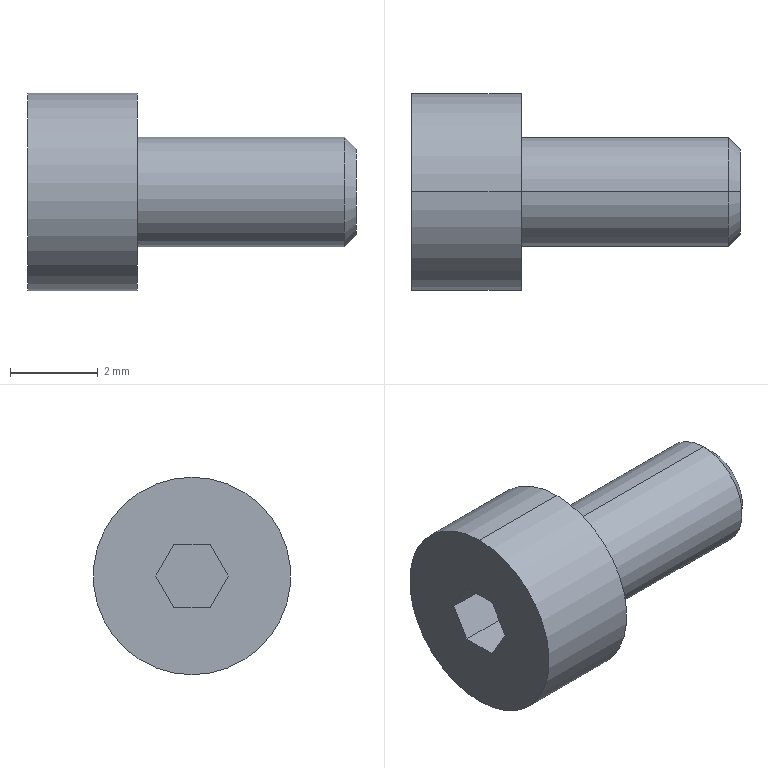Part | STEP file | _DBA11-D25-d10-e12-005.stp | 1 solid | 16 faces | box 7.5 x 4.5 x 4.5 mm | volume 61.818 mm3 | plane 10 | cylinder 4 | cone 2 | commonest cylinder face diameters 2.5 x2 4.5 x2
STEP:
#1=CARTESIAN_POINT('',(2.5,0.,-1.25));
#2=VERTEX_POINT('',#1);
#3=CARTESIAN_POINT('',(2.5,0.,1.25));
#4=VERTEX_POINT('',#3);
#5=CARTESIAN_POINT('',(2.5,0.,0.));
#6=DIRECTION('',(-1.,0.,0.));
#7=DIRECTION('',(0.,0.,1.));
#8=AXIS2_PLACEMENT_3D('',#5,#6,#7);
#9=CIRCLE('',#8,1.25);
#10=EDGE_CURVE('',#2,#4,#9,.T.);
#11=ORIENTED_EDGE('',*,*,#10,.F.);
#12=CARTESIAN_POINT('',(7.224,0.,-1.25));
#13=VERTEX_POINT('',#12);
#14=CARTESIAN_POINT('',(0.,0.,-1.25));
#15=DIRECTION('',(1.,0.,0.));
#16=VECTOR('',#15,1000.);
#17=LINE('',#14,#16);
#18=EDGE_CURVE('',#2,#13,#17,.T.);
#19=ORIENTED_EDGE('',*,*,#18,.T.);
#20=CARTESIAN_POINT('',(7.224,0.,1.25));
#21=VERTEX_POINT('',#20);
#22=CARTESIAN_POINT('',(7.224,0.,0.));
#23=DIRECTION('',(-1.,0.,0.));
#24=DIRECTION('',(0.,0.,1.));
#25=AXIS2_PLACEMENT_3D('',#22,#23,#24);
#26=CIRCLE('',#25,1.25);
#27=EDGE_CURVE('',#13,#21,#26,.T.);
#28=ORIENTED_EDGE('',*,*,#27,.T.);
#29=CARTESIAN_POINT('',(0.,0.,1.25));
#30=DIRECTION('',(1.,0.,0.));
#31=VECTOR('',#30,1000.);
#32=LINE('',#29,#31);
#33=EDGE_CURVE('',#4,#21,#32,.T.);
#34=ORIENTED_EDGE('',*,*,#33,.F.);
#35=EDGE_LOOP('',(#11,#19,#28,#34));
#36=FACE_OUTER_BOUND('',#35,.T.);
#37=CARTESIAN_POINT('',(0.,0.,0.));
#38=DIRECTION('',(1.,0.,0.));
#39=DIRECTION('',(0.,0.,1.));
#40=AXIS2_PLACEMENT_3D('',#37,#38,#39);
#41=CYLINDRICAL_SURFACE('',#40,1.25);
#42=ADVANCED_FACE('',(#36),#41,.T.);
#43=CARTESIAN_POINT('',(0.,0.,-2.25));
#44=VERTEX_POINT('',#43);
#45=CARTESIAN_POINT('',(0.,0.,2.25));
#46=VERTEX_POINT('',#45);
#47=CARTESIAN_POINT('',(0.,0.,0.));
#48=DIRECTION('',(-1.,0.,0.));
#49=DIRECTION('',(0.,0.,1.));
#50=AXIS2_PLACEMENT_3D('',#47,#48,#49);
#51=CIRCLE('',#50,2.25);
#52=EDGE_CURVE('',#44,#46,#51,.T.);
#53=ORIENTED_EDGE('',*,*,#52,.F.);
#54=CARTESIAN_POINT('',(2.5,0.,-2.25));
#55=VERTEX_POINT('',#54);
#56=CARTESIAN_POINT('',(0.,0.,-2.25));
#57=DIRECTION('',(1.,0.,0.));
#58=VECTOR('',#57,1000.);
#59=LINE('',#56,#58);
#60=EDGE_CURVE('',#44,#55,#59,.T.);
#61=ORIENTED_EDGE('',*,*,#60,.T.);
#62=CARTESIAN_POINT('',(2.5,0.,2.25));
#63=VERTEX_POINT('',#62);
#64=CARTESIAN_POINT('',(2.5,0.,0.));
#65=DIRECTION('',(-1.,0.,0.));
#66=DIRECTION('',(0.,0.,1.));
#67=AXIS2_PLACEMENT_3D('',#64,#65,#66);
#68=CIRCLE('',#67,2.25);
#69=EDGE_CURVE('',#55,#63,#68,.T.);
#70=ORIENTED_EDGE('',*,*,#69,.T.);
#71=CARTESIAN_POINT('',(0.,0.,2.25));
#72=DIRECTION('',(1.,0.,0.));
#73=VECTOR('',#72,1000.);
#74=LINE('',#71,#73);
#75=EDGE_CURVE('',#46,#63,#74,.T.);
#76=ORIENTED_EDGE('',*,*,#75,.F.);
#77=EDGE_LOOP('',(#53,#61,#70,#76));
#78=FACE_OUTER_BOUND('',#77,.T.);
#79=CARTESIAN_POINT('',(0.,0.,0.));
#80=DIRECTION('',(1.,0.,0.));
#81=DIRECTION('',(0.,0.,1.));
#82=AXIS2_PLACEMENT_3D('',#79,#80,#81);
#83=CYLINDRICAL_SURFACE('',#82,2.25);
#84=ADVANCED_FACE('',(#78),#83,.T.);
#85=CARTESIAN_POINT('',(7.5,0.,0.974));
#86=VERTEX_POINT('',#85);
#87=CARTESIAN_POINT('',(7.5,0.,-0.974));
#88=VERTEX_POINT('',#87);
#89=CARTESIAN_POINT('',(7.5,0.,0.));
#90=DIRECTION('',(-1.,0.,0.));
#91=DIRECTION('',(0.,0.,1.));
#92=AXIS2_PLACEMENT_3D('',#89,#90,#91);
#93=CIRCLE('',#92,0.974);
#94=EDGE_CURVE('',#86,#88,#93,.T.);
#95=ORIENTED_EDGE('',*,*,#94,.T.);
#96=CARTESIAN_POINT('',(7.5,0.,-0.974));
#97=DIRECTION('',(-0.7071,0.,-0.7071));
#98=VECTOR('',#97,1000.);
#99=LINE('',#96,#98);
#100=EDGE_CURVE('',#88,#13,#99,.T.);
#101=ORIENTED_EDGE('',*,*,#100,.T.);
#102=CARTESIAN_POINT('',(7.224,0.,0.));
#103=DIRECTION('',(-1.,0.,0.));
#104=DIRECTION('',(0.,0.,1.));
#105=AXIS2_PLACEMENT_3D('',#102,#103,#104);
#106=CIRCLE('',#105,1.25);
#107=EDGE_CURVE('',#21,#13,#106,.T.);
#108=ORIENTED_EDGE('',*,*,#107,.F.);
#109=CARTESIAN_POINT('',(7.5,0.,0.974));
#110=DIRECTION('',(-0.7071,0.,0.7071));
#111=VECTOR('',#110,1000.);
#112=LINE('',#109,#111);
#113=EDGE_CURVE('',#86,#21,#112,.T.);
#114=ORIENTED_EDGE('',*,*,#113,.F.);
#115=EDGE_LOOP('',(#95,#101,#108,#114));
#116=FACE_OUTER_BOUND('',#115,.T.);
#117=CARTESIAN_POINT('',(7.5,0.,0.));
#118=DIRECTION('',(-1.,0.,0.));
#119=DIRECTION('',(0.,0.,1.));
#120=AXIS2_PLACEMENT_3D('',#117,#118,#119);
#121=CONICAL_SURFACE('',#120,0.974,0.7854);
#122=ADVANCED_FACE('',(#116),#121,.T.);
#123=ORIENTED_EDGE('',*,*,#100,.F.);
#124=CARTESIAN_POINT('',(7.5,0.,0.));
#125=DIRECTION('',(-1.,0.,0.));
#126=DIRECTION('',(0.,0.,1.));
#127=AXIS2_PLACEMENT_3D('',#124,#125,#126);
#128=CIRCLE('',#127,0.974);
#129=EDGE_CURVE('',#88,#86,#128,.T.);
#130=ORIENTED_EDGE('',*,*,#129,.T.);
#131=ORIENTED_EDGE('',*,*,#113,.T.);
#132=ORIENTED_EDGE('',*,*,#27,.F.);
#133=EDGE_LOOP('',(#123,#130,#131,#132));
#134=FACE_OUTER_BOUND('',#133,.T.);
#135=CARTESIAN_POINT('',(7.5,0.,0.));
#136=DIRECTION('',(-1.,0.,0.));
#137=DIRECTION('',(0.,0.,1.));
#138=AXIS2_PLACEMENT_3D('',#135,#136,#137);
#139=CONICAL_SURFACE('',#138,0.974,0.7854);
#140=ADVANCED_FACE('',(#134),#139,.T.);
#141=ORIENTED_EDGE('',*,*,#94,.F.);
#142=ORIENTED_EDGE('',*,*,#129,.F.);
#143=EDGE_LOOP('',(#141,#142));
#144=FACE_OUTER_BOUND('',#143,.T.);
#145=CARTESIAN_POINT('',(7.5,0.,0.));
#146=DIRECTION('',(-1.,0.,0.));
#147=DIRECTION('',(0.,0.,1.));
#148=AXIS2_PLACEMENT_3D('',#145,#146,#147);
#149=PLANE('',#148);
#150=ADVANCED_FACE('',(#144),#149,.F.);
#151=CARTESIAN_POINT('',(0.,0.,0.));
#152=DIRECTION('',(-1.,0.,0.));
#153=DIRECTION('',(0.,0.,1.));
#154=AXIS2_PLACEMENT_3D('',#151,#152,#153);
#155=CIRCLE('',#154,2.25);
#156=EDGE_CURVE('',#46,#44,#155,.T.);
#157=ORIENTED_EDGE('',*,*,#156,.T.);
#158=ORIENTED_EDGE('',*,*,#52,.T.);
#159=EDGE_LOOP('',(#157,#158));
#160=FACE_OUTER_BOUND('',#159,.T.);
#161=CARTESIAN_POINT('',(0.,-0.4124,0.7143));
#162=VERTEX_POINT('',#161);
#163=CARTESIAN_POINT('',(0.,-0.8248,0.));
#164=VERTEX_POINT('',#163);
#165=CARTESIAN_POINT('',(0.,-0.4124,0.7143));
#166=DIRECTION('',(0.,-0.5,-0.866));
#167=VECTOR('',#166,1000.);
#168=LINE('',#165,#167);
#169=EDGE_CURVE('',#162,#164,#168,.T.);
#170=ORIENTED_EDGE('',*,*,#169,.T.);
#171=CARTESIAN_POINT('',(0.,-0.4124,-0.7143));
#172=VERTEX_POINT('',#171);
#173=CARTESIAN_POINT('',(0.,-0.8248,0.));
#174=DIRECTION('',(0.,0.5,-0.866));
#175=VECTOR('',#174,1000.);
#176=LINE('',#173,#175);
#177=EDGE_CURVE('',#164,#172,#176,.T.);
#178=ORIENTED_EDGE('',*,*,#177,.T.);
#179=CARTESIAN_POINT('',(0.,0.4124,-0.7143));
#180=VERTEX_POINT('',#179);
#181=CARTESIAN_POINT('',(0.,-0.4124,-0.7143));
#182=DIRECTION('',(0.,1.,0.));
#183=VECTOR('',#182,1000.);
#184=LINE('',#181,#183);
#185=EDGE_CURVE('',#172,#180,#184,.T.);
#186=ORIENTED_EDGE('',*,*,#185,.T.);
#187=CARTESIAN_POINT('',(0.,0.8248,0.));
#188=VERTEX_POINT('',#187);
#189=CARTESIAN_POINT('',(0.,0.4124,-0.7143));
#190=DIRECTION('',(0.,0.5,0.866));
#191=VECTOR('',#190,1000.);
#192=LINE('',#189,#191);
#193=EDGE_CURVE('',#180,#188,#192,.T.);
#194=ORIENTED_EDGE('',*,*,#193,.T.);
#195=CARTESIAN_POINT('',(0.,0.4124,0.7143));
#196=VERTEX_POINT('',#195);
#197=CARTESIAN_POINT('',(0.,0.8248,0.));
#198=DIRECTION('',(0.,-0.5,0.866));
#199=VECTOR('',#198,1000.);
#200=LINE('',#197,#199);
#201=EDGE_CURVE('',#188,#196,#200,.T.);
#202=ORIENTED_EDGE('',*,*,#201,.T.);
#203=CARTESIAN_POINT('',(0.,0.4124,0.7143));
#204=DIRECTION('',(0.,-1.,0.));
#205=VECTOR('',#204,1000.);
#206=LINE('',#203,#205);
#207=EDGE_CURVE('',#196,#162,#206,.T.);
#208=ORIENTED_EDGE('',*,*,#207,.T.);
#209=EDGE_LOOP('',(#170,#178,#186,#194,#202,#208));
#210=FACE_BOUND('',#209,.T.);
#211=CARTESIAN_POINT('',(0.,-2.25,0.));
#212=DIRECTION('',(1.,0.,0.));
#213=DIRECTION('',(0.,1.,0.));
#214=AXIS2_PLACEMENT_3D('',#211,#212,#213);
#215=PLANE('',#214);
#216=ADVANCED_FACE('',(#160,#210),#215,.F.);
#217=ORIENTED_EDGE('',*,*,#60,.F.);
#218=ORIENTED_EDGE('',*,*,#156,.F.);
#219=ORIENTED_EDGE('',*,*,#75,.T.);
#220=CARTESIAN_POINT('',(2.5,0.,0.));
#221=DIRECTION('',(-1.,0.,0.));
#222=DIRECTION('',(0.,0.,1.));
#223=AXIS2_PLACEMENT_3D('',#220,#221,#222);
#224=CIRCLE('',#223,2.25);
#225=EDGE_CURVE('',#63,#55,#224,.T.);
#226=ORIENTED_EDGE('',*,*,#225,.T.);
#227=EDGE_LOOP('',(#217,#218,#219,#226));
#228=FACE_OUTER_BOUND('',#227,.T.);
#229=CARTESIAN_POINT('',(0.,0.,0.));
#230=DIRECTION('',(1.,0.,0.));
#231=DIRECTION('',(0.,0.,1.));
#232=AXIS2_PLACEMENT_3D('',#229,#230,#231);
#233=CYLINDRICAL_SURFACE('',#232,2.25);
#234=ADVANCED_FACE('',(#228),#233,.T.);
#235=ORIENTED_EDGE('',*,*,#225,.F.);
#236=ORIENTED_EDGE('',*,*,#69,.F.);
#237=EDGE_LOOP('',(#235,#236));
#238=FACE_OUTER_BOUND('',#237,.T.);
#239=CARTESIAN_POINT('',(2.5,0.,0.));
#240=DIRECTION('',(-1.,0.,0.));
#241=DIRECTION('',(0.,0.,1.));
#242=AXIS2_PLACEMENT_3D('',#239,#240,#241);
#243=CIRCLE('',#242,1.25);
#244=EDGE_CURVE('',#4,#2,#243,.T.);
#245=ORIENTED_EDGE('',*,*,#244,.T.);
#246=ORIENTED_EDGE('',*,*,#10,.T.);
#247=EDGE_LOOP('',(#245,#246));
#248=FACE_BOUND('',#247,.T.);
#249=CARTESIAN_POINT('',(2.5,-1.25,0.));
#250=DIRECTION('',(-1.,0.,0.));
#251=DIRECTION('',(0.,0.,1.));
#252=AXIS2_PLACEMENT_3D('',#249,#250,#251);
#253=PLANE('',#252);
#254=ADVANCED_FACE('',(#238,#248),#253,.F.);
#255=ORIENTED_EDGE('',*,*,#18,.F.);
#256=ORIENTED_EDGE('',*,*,#244,.F.);
#257=ORIENTED_EDGE('',*,*,#33,.T.);
#258=ORIENTED_EDGE('',*,*,#107,.T.);
#259=EDGE_LOOP('',(#255,#256,#257,#258));
#260=FACE_OUTER_BOUND('',#259,.T.);
#261=CARTESIAN_POINT('',(0.,0.,0.));
#262=DIRECTION('',(1.,0.,0.));
#263=DIRECTION('',(0.,0.,1.));
#264=AXIS2_PLACEMENT_3D('',#261,#262,#263);
#265=CYLINDRICAL_SURFACE('',#264,1.25);
#266=ADVANCED_FACE('',(#260),#265,.T.);
#267=ORIENTED_EDGE('',*,*,#207,.F.);
#268=CARTESIAN_POINT('',(1.25,0.4124,0.7143));
#269=VERTEX_POINT('',#268);
#270=CARTESIAN_POINT('',(1.25,0.4124,0.7143));
#271=DIRECTION('',(-1.,0.,0.));
#272=VECTOR('',#271,1000.);
#273=LINE('',#270,#272);
#274=EDGE_CURVE('',#269,#196,#273,.T.);
#275=ORIENTED_EDGE('',*,*,#274,.F.);
#276=CARTESIAN_POINT('',(1.25,-0.4124,0.7143));
#277=VERTEX_POINT('',#276);
#278=CARTESIAN_POINT('',(1.25,0.4124,0.7143));
#279=DIRECTION('',(0.,-1.,0.));
#280=VECTOR('',#279,1000.);
#281=LINE('',#278,#280);
#282=EDGE_CURVE('',#269,#277,#281,.T.);
#283=ORIENTED_EDGE('',*,*,#282,.T.);
#284=CARTESIAN_POINT('',(1.25,-0.4124,0.7143));
#285=DIRECTION('',(-1.,0.,0.));
#286=VECTOR('',#285,1000.);
#287=LINE('',#284,#286);
#288=EDGE_CURVE('',#277,#162,#287,.T.);
#289=ORIENTED_EDGE('',*,*,#288,.T.);
#290=EDGE_LOOP('',(#267,#275,#283,#289));
#291=FACE_OUTER_BOUND('',#290,.T.);
#292=CARTESIAN_POINT('',(1.25,0.4124,0.7143));
#293=DIRECTION('',(0.,0.,-1.));
#294=DIRECTION('',(0.,-1.,0.));
#295=AXIS2_PLACEMENT_3D('',#292,#293,#294);
#296=PLANE('',#295);
#297=ADVANCED_FACE('',(#291),#296,.T.);
#298=ORIENTED_EDGE('',*,*,#169,.F.);
#299=ORIENTED_EDGE('',*,*,#288,.F.);
#300=CARTESIAN_POINT('',(1.25,-0.8248,0.));
#301=VERTEX_POINT('',#300);
#302=CARTESIAN_POINT('',(1.25,-0.4124,0.7143));
#303=DIRECTION('',(0.,-0.5,-0.866));
#304=VECTOR('',#303,1000.);
#305=LINE('',#302,#304);
#306=EDGE_CURVE('',#277,#301,#305,.T.);
#307=ORIENTED_EDGE('',*,*,#306,.T.);
#308=CARTESIAN_POINT('',(1.25,-0.8248,0.));
#309=DIRECTION('',(-1.,0.,0.));
#310=VECTOR('',#309,1000.);
#311=LINE('',#308,#310);
#312=EDGE_CURVE('',#301,#164,#311,.T.);
#313=ORIENTED_EDGE('',*,*,#312,.T.);
#314=EDGE_LOOP('',(#298,#299,#307,#313));
#315=FACE_OUTER_BOUND('',#314,.T.);
#316=CARTESIAN_POINT('',(1.25,-0.4124,0.7143));
#317=DIRECTION('',(0.,0.866,-0.5));
#318=DIRECTION('',(-1.,0.,0.));
#319=AXIS2_PLACEMENT_3D('',#316,#317,#318);
#320=PLANE('',#319);
#321=ADVANCED_FACE('',(#315),#320,.T.);
#322=ORIENTED_EDGE('',*,*,#177,.F.);
#323=ORIENTED_EDGE('',*,*,#312,.F.);
#324=CARTESIAN_POINT('',(1.25,-0.4124,-0.7143));
#325=VERTEX_POINT('',#324);
#326=CARTESIAN_POINT('',(1.25,-0.8248,0.));
#327=DIRECTION('',(0.,0.5,-0.866));
#328=VECTOR('',#327,1000.);
#329=LINE('',#326,#328);
#330=EDGE_CURVE('',#301,#325,#329,.T.);
#331=ORIENTED_EDGE('',*,*,#330,.T.);
#332=CARTESIAN_POINT('',(1.25,-0.4124,-0.7143));
#333=DIRECTION('',(-1.,0.,0.));
#334=VECTOR('',#333,1000.);
#335=LINE('',#332,#334);
#336=EDGE_CURVE('',#325,#172,#335,.T.);
#337=ORIENTED_EDGE('',*,*,#336,.T.);
#338=EDGE_LOOP('',(#322,#323,#331,#337));
#339=FACE_OUTER_BOUND('',#338,.T.);
#340=CARTESIAN_POINT('',(1.25,-0.8248,0.));
#341=DIRECTION('',(0.,0.866,0.5));
#342=DIRECTION('',(1.,0.,0.));
#343=AXIS2_PLACEMENT_3D('',#340,#341,#342);
#344=PLANE('',#343);
#345=ADVANCED_FACE('',(#339),#344,.T.);
#346=ORIENTED_EDGE('',*,*,#185,.F.);
#347=ORIENTED_EDGE('',*,*,#336,.F.);
#348=CARTESIAN_POINT('',(1.25,0.4124,-0.7143));
#349=VERTEX_POINT('',#348);
#350=CARTESIAN_POINT('',(1.25,-0.4124,-0.7143));
#351=DIRECTION('',(0.,1.,0.));
#352=VECTOR('',#351,1000.);
#353=LINE('',#350,#352);
#354=EDGE_CURVE('',#325,#349,#353,.T.);
#355=ORIENTED_EDGE('',*,*,#354,.T.);
#356=CARTESIAN_POINT('',(1.25,0.4124,-0.7143));
#357=DIRECTION('',(-1.,0.,0.));
#358=VECTOR('',#357,1000.);
#359=LINE('',#356,#358);
#360=EDGE_CURVE('',#349,#180,#359,.T.);
#361=ORIENTED_EDGE('',*,*,#360,.T.);
#362=EDGE_LOOP('',(#346,#347,#355,#361));
#363=FACE_OUTER_BOUND('',#362,.T.);
#364=CARTESIAN_POINT('',(1.25,-0.4124,-0.7143));
#365=DIRECTION('',(0.,0.,1.));
#366=DIRECTION('',(1.,0.,0.));
#367=AXIS2_PLACEMENT_3D('',#364,#365,#366);
#368=PLANE('',#367);
#369=ADVANCED_FACE('',(#363),#368,.T.);
#370=ORIENTED_EDGE('',*,*,#193,.F.);
#371=ORIENTED_EDGE('',*,*,#360,.F.);
#372=CARTESIAN_POINT('',(1.25,0.8248,0.));
#373=VERTEX_POINT('',#372);
#374=CARTESIAN_POINT('',(1.25,0.4124,-0.7143));
#375=DIRECTION('',(0.,0.5,0.866));
#376=VECTOR('',#375,1000.);
#377=LINE('',#374,#376);
#378=EDGE_CURVE('',#349,#373,#377,.T.);
#379=ORIENTED_EDGE('',*,*,#378,.T.);
#380=CARTESIAN_POINT('',(1.25,0.8248,0.));
#381=DIRECTION('',(-1.,0.,0.));
#382=VECTOR('',#381,1000.);
#383=LINE('',#380,#382);
#384=EDGE_CURVE('',#373,#188,#383,.T.);
#385=ORIENTED_EDGE('',*,*,#384,.T.);
#386=EDGE_LOOP('',(#370,#371,#379,#385));
#387=FACE_OUTER_BOUND('',#386,.T.);
#388=CARTESIAN_POINT('',(1.25,0.4124,-0.7143));
#389=DIRECTION('',(0.,-0.866,0.5));
#390=DIRECTION('',(-1.,0.,0.));
#391=AXIS2_PLACEMENT_3D('',#388,#389,#390);
#392=PLANE('',#391);
#393=ADVANCED_FACE('',(#387),#392,.T.);
#394=ORIENTED_EDGE('',*,*,#201,.F.);
#395=ORIENTED_EDGE('',*,*,#384,.F.);
#396=CARTESIAN_POINT('',(1.25,0.8248,0.));
#397=DIRECTION('',(0.,-0.5,0.866));
#398=VECTOR('',#397,1000.);
#399=LINE('',#396,#398);
#400=EDGE_CURVE('',#373,#269,#399,.T.);
#401=ORIENTED_EDGE('',*,*,#400,.T.);
#402=ORIENTED_EDGE('',*,*,#274,.T.);
#403=EDGE_LOOP('',(#394,#395,#401,#402));
#404=FACE_OUTER_BOUND('',#403,.T.);
#405=CARTESIAN_POINT('',(1.25,0.8248,0.));
#406=DIRECTION('',(0.,-0.866,-0.5));
#407=DIRECTION('',(0.,0.5,-0.866));
#408=AXIS2_PLACEMENT_3D('',#405,#406,#407);
#409=PLANE('',#408);
#410=ADVANCED_FACE('',(#404),#409,.T.);
#411=ORIENTED_EDGE('',*,*,#282,.F.);
#412=ORIENTED_EDGE('',*,*,#400,.F.);
#413=ORIENTED_EDGE('',*,*,#378,.F.);
#414=ORIENTED_EDGE('',*,*,#354,.F.);
#415=ORIENTED_EDGE('',*,*,#330,.F.);
#416=ORIENTED_EDGE('',*,*,#306,.F.);
#417=EDGE_LOOP('',(#411,#412,#413,#414,#415,#416));
#418=FACE_OUTER_BOUND('',#417,.T.);
#419=CARTESIAN_POINT('',(1.25,0.,0.));
#420=DIRECTION('',(1.,0.,0.));
#421=DIRECTION('',(0.,1.,0.));
#422=AXIS2_PLACEMENT_3D('',#419,#420,#421);
#423=PLANE('',#422);
#424=ADVANCED_FACE('',(#418),#423,.F.);
#425=CLOSED_SHELL('',(#42,#84,#122,#140,#150,#216,#234,#254,#266,#297,#321,#345,#369,#393,#410,#424));
#426=MANIFOLD_SOLID_BREP('',#425);
#427=CARTESIAN_POINT('',(0.,0.,0.));
#428=DIRECTION('',(0.,0.,1.));
#429=DIRECTION('',(1.,0.,0.));
#430=AXIS2_PLACEMENT_3D('',#427,#428,#429);
#431=(LENGTH_UNIT()NAMED_UNIT(*)SI_UNIT(.MILLI.,.METRE.));
#432=UNCERTAINTY_MEASURE_WITH_UNIT(LENGTH_MEASURE(0.00001),#431,'','');
#433=(NAMED_UNIT(*)PLANE_ANGLE_UNIT()SI_UNIT($,.RADIAN.));
#434=(NAMED_UNIT(*)SI_UNIT($,.STERADIAN.)SOLID_ANGLE_UNIT());
#435=(GEOMETRIC_REPRESENTATION_CONTEXT(3)GLOBAL_UNCERTAINTY_ASSIGNED_CONTEXT((#432))GLOBAL_UNIT_ASSIGNED_CONTEXT((#431,#433,#434))REPRESENTATION_CONTEXT('',''));
#436=ADVANCED_BREP_SHAPE_REPRESENTATION('',(#426,#430),#435);